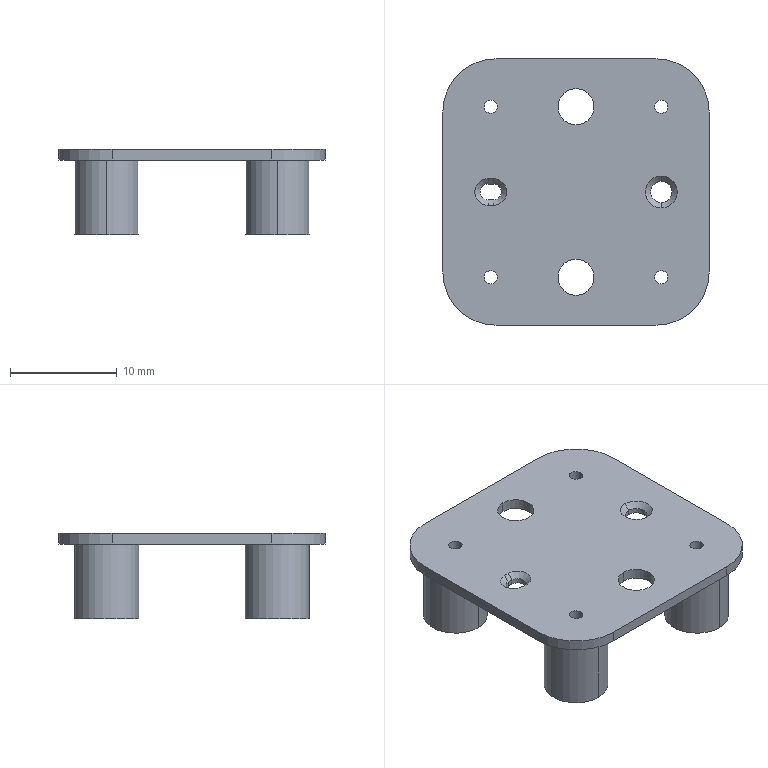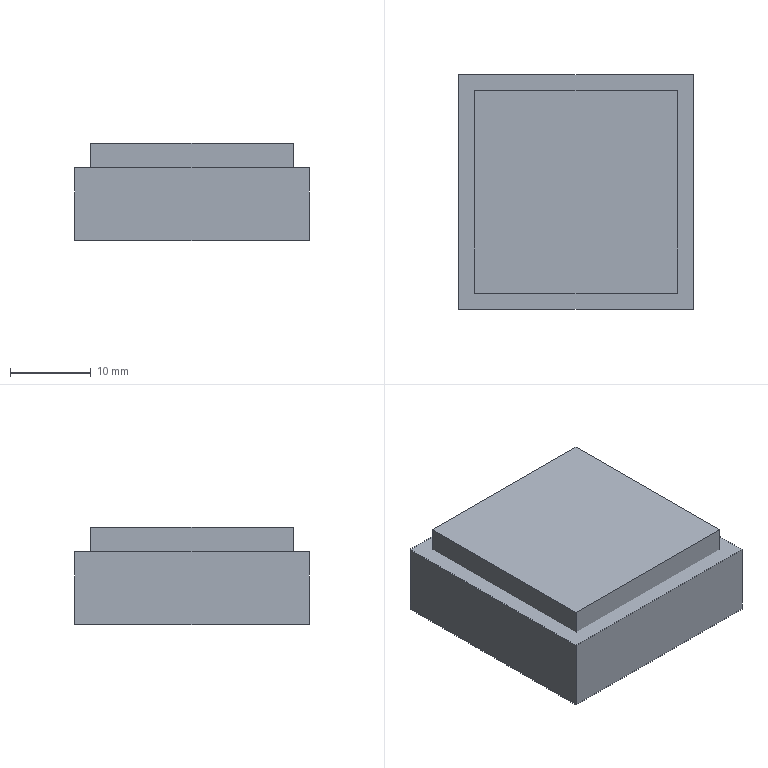CAM job | NX | 3-axis milling, drilling | part box 25 x 25 x 8 mm | stock box 29 x 29 x 12 mm
Tools:
number,name,description,diameter,corner_radius,flute_length,length,flutes
19,D80,Milling Tool-5 Parameters,80.0,0.0,50.0,75.0,2
1,D6A45,Milling Tool-5 Parameters,6.0,0.0,50.0,75.0,2
20,1.25ZT,Drilling Tool,1.25,0.0,35.0,50.0,2
3,3.4ZT,Drilling Tool,3.4,0.0,35.0,50.0,2
18,D1.0,Milling Tool-5 Parameters,1.0,0.0,50.0,75.0,2
15,D10,Milling Tool-5 Parameters,10.0,0.0,50.0,75.0,2
11,D4,Milling Tool-5 Parameters,4.0,0.0,50.0,75.0,2
14,D10JING,Milling Tool-5 Parameters,10.0,0.0,50.0,75.0,2
Operations:
program,operation,operation_type,tool,method,geometry_group,spindle_rpm,surface_speed,feed_per_tooth,feed_cut,feed_plunge,cut_length_mm,path_length_mm,cut_time_min,machine_time_min
1,FLOOR_WALL_COPY,VolumeBased25DMillingOperation,D80,METHOD,A,6500.0,1633.0,0.1154,1500.0,100.0,125.0,179.0,0.0833,0.0887
1,DRILLING_COPY_1,Operation,D6A45,METHOD,A,5000.0,94.0,0.035,350.0,0.0,26.25,181.764,0.075,0.0906
1,DRILLING_COPY_1_COPY_COPY,Operation,1.25ZT,METHOD,A,2000.0,7.0,0.03,120.0,0.0,49.502,216.841,0.4125,0.4293
1,DRILLING_COPY_1_COPY_1_1_COPY_1,Operation,3.4ZT,METHOD,A,2000.0,34.0,0.05,200.0,0.0,13.043,105.365,0.0652,0.0744
1,ZLEVEL_PROFILE_COPY,ZLevelMilling,D1.0,METHOD,A,9500.0,44.0,0.0526,1000.0,1000.0,84.046,219.2,0.084,0.0976
1,ZLEVEL_PROFILE,ZLevelMilling,D10,METHOD,A,9500.0,298.0,0.1684,3200.0,1000.0,1094.287,1159.287,0.3748,0.3813
1,ZLEVEL_PROFILE_COPY_1_COPY_COPY_1_COPY_COPY,ZLevelMilling,D10JING,METHOD,A,9500.0,298.0,0.0632,1200.0,1000.0,126.091,200.091,0.1053,0.1127
1,PLANAR_MILL_COPY_COPY_COPY_COPY_COPY_COPY_1_COPY_1,PlanarMilling,D6A45,METHOD,A,9500.0,179.0,0.0658,1250.0,100.0,125.721,401.416,0.1006,0.1281
1,PLANAR_MILL_COPY_COPY_COPY_COPY_COPY_COPY_1_COPY_1_COPY,PlanarMilling,D6A45,METHOD,A,9500.0,179.0,0.0658,1250.0,100.0,13.807,146.943,0.011,0.0244
2,FLOOR_WALL_COPY_COPY,VolumeBased25DMillingOperation,D80,METHOD,B,6500.0,1633.0,0.1154,1500.0,100.0,484.0,1033.001,0.3227,0.3776
2,FLOOR_WALL,VolumeBased25DMillingOperation,D4,METHOD,B,9500.0,0.0,0.0,2000.0,1000.0,8275.803,8426.953,4.16,4.175
2,FLOOR_WALL_COPY_1,VolumeBased25DMillingOperation,D4,METHOD,B,9500.0,179.0,0.0579,1100.0,100.0,473.928,1300.321,0.4308,0.5135
2,HOLE_MILLING,CylinderMilling,D1.0,METHOD,B,9500.0,29.0,0.0421,800.0,100.0,627.957,928.758,0.7849,0.815
2,DRILLING_COPY_1_COPY,Operation,D6A45,METHOD,B,5000.0,94.0,0.035,350.0,0.0,17.6,153.036,0.0503,0.0638
2,PLANAR_MILL_COPY_COPY_COPY_COPY_COPY_COPY_1_COPY_1_COPY_1,PlanarMilling,D6A45,METHOD,B,9500.0,179.0,0.0658,1250.0,100.0,115.882,398.337,0.0927,0.121
2,ZLEVEL_PROFILE_COPY_1_COPY_COPY_1_COPY_COPY_1,ZLevelMilling,D4,METHOD,B,9500.0,298.0,0.0632,1200.0,1000.0,109.115,182.915,0.0913,0.0987